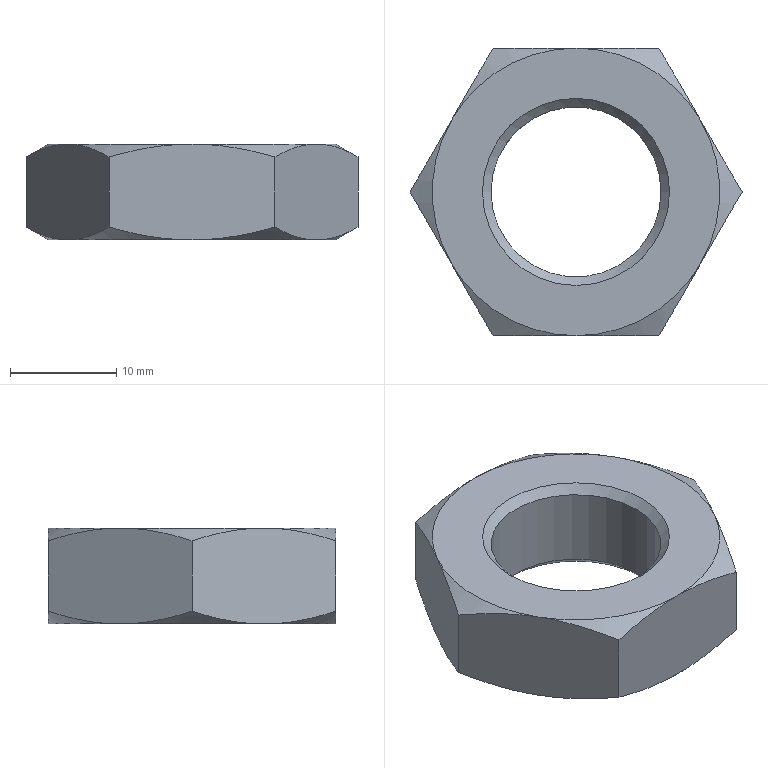Part | STEP file | YBQDJ-PD-21 | 1 solid | 23 faces | box 31.177 x 27 x 9 mm | volume 3802 mm3 | cone 14 | plane 8 | cylinder 1 | commonest cylinder face diameters 15.97 x1